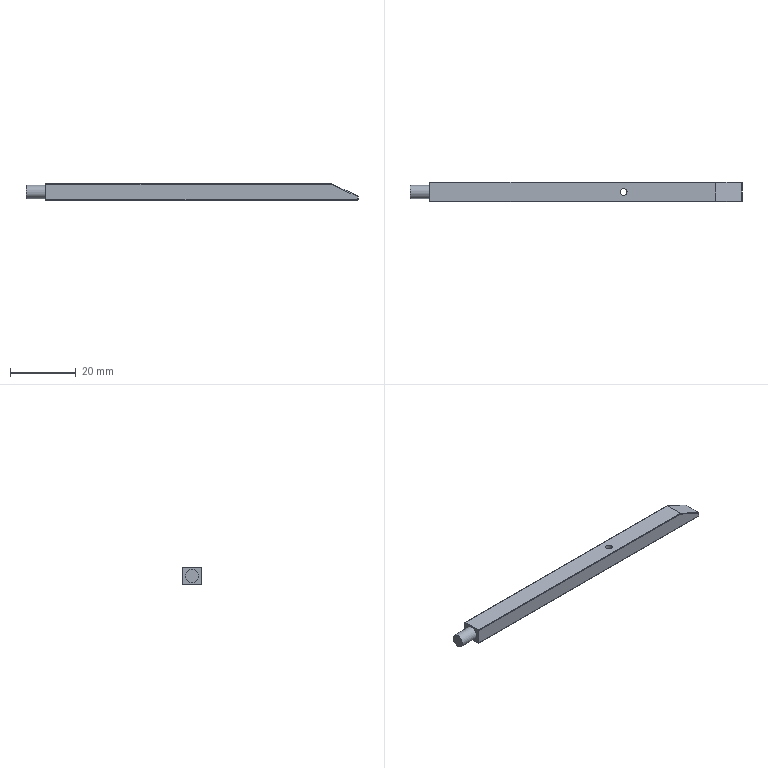Part | STEP file | 1-08.2 | 1 solid | 24 faces | box 101 x 6 x 5 mm | volume 2812 mm3 | plane 22 | cylinder 2 | commonest cylinder face diameters 2 x1 4 x1
STEP:
#1=CARTESIAN_POINT('',(0.,0.,0.));
#2=DIRECTION('',(0.,0.,1.));
#3=DIRECTION('',(1.,0.,0.));
#4=AXIS2_PLACEMENT_3D('',#1,#2,#3);
#5=CARTESIAN_POINT('',(-43.5,-2.,0.));
#6=VERTEX_POINT('',#5);
#7=CARTESIAN_POINT('',(-43.5,0.,0.));
#8=DIRECTION('',(-1.,0.,0.));
#9=DIRECTION('',(0.,-1.,0.));
#10=AXIS2_PLACEMENT_3D('',#7,#8,#9);
#11=CIRCLE('',#10,2.);
#12=CARTESIAN_POINT('',(-43.5,0.,0.));
#13=DIRECTION('',(-1.,0.,0.));
#14=DIRECTION('',(0.,-1.,0.));
#15=AXIS2_PLACEMENT_3D('',#12,#13,#14);
#16=CYLINDRICAL_SURFACE('',#15,2.);
#17=CARTESIAN_POINT('',(0.,0.));
#18=DIRECTION('',(1.,0.));
#19=VECTOR('',#18,1.);
#20=LINE('',#17,#19);
#21=(GEOMETRIC_REPRESENTATION_CONTEXT(2)PARAMETRIC_REPRESENTATION_CONTEXT()REPRESENTATION_CONTEXT('',''));
#22=DEFINITIONAL_REPRESENTATION('',(#20),#21);
#23=PCURVE('',#16,#22);
#24=CARTESIAN_POINT('',(-43.5,0.,0.));
#25=DIRECTION('',(1.,0.,0.));
#26=DIRECTION('',(0.,0.,-1.));
#27=AXIS2_PLACEMENT_3D('',#24,#25,#26);
#28=PLANE('',#27);
#29=CARTESIAN_POINT('',(0.,-2.));
#30=CARTESIAN_POINT('',(-3.464,-2.));
#31=CARTESIAN_POINT('',(-1.732,1.));
#32=CARTESIAN_POINT('',(0.,4.));
#33=CARTESIAN_POINT('',(1.732,1.));
#34=CARTESIAN_POINT('',(3.464,-2.));
#35=CARTESIAN_POINT('',(0.,-2.));
#36=(BOUNDED_CURVE()B_SPLINE_CURVE(2,(#29,#30,#31,#32,#33,#34,#35),.UNSPECIFIED.,.T.,.F.)B_SPLINE_CURVE_WITH_KNOTS((1,2,2,2,2,1),(-2.094,0.,2.094,4.189,6.283,8.378),.UNSPECIFIED.)CURVE()GEOMETRIC_REPRESENTATION_ITEM()RATIONAL_B_SPLINE_CURVE((1.,0.5,1.,0.5,1.,0.5,1.))REPRESENTATION_ITEM(''));
#37=(GEOMETRIC_REPRESENTATION_CONTEXT(2)PARAMETRIC_REPRESENTATION_CONTEXT()REPRESENTATION_CONTEXT('',''));
#38=DEFINITIONAL_REPRESENTATION('',(#36),#37);
#39=PCURVE('',#28,#38);
#40=SURFACE_CURVE('',#11,(#23,#39),.PCURVE_S1.);
#41=EDGE_CURVE('',#6,#6,#40,.T.);
#42=ORIENTED_EDGE('',*,*,#41,.T.);
#43=CARTESIAN_POINT('',(-49.5,-2.,0.));
#44=VERTEX_POINT('',#43);
#45=CARTESIAN_POINT('',(-43.5,-2.,0.));
#46=DIRECTION('',(-1.,0.,0.));
#47=VECTOR('',#46,1.);
#48=LINE('',#45,#47);
#49=CARTESIAN_POINT('',(6.283,0.));
#50=DIRECTION('',(0.,1.));
#51=VECTOR('',#50,1.);
#52=LINE('',#49,#51);
#53=(GEOMETRIC_REPRESENTATION_CONTEXT(2)PARAMETRIC_REPRESENTATION_CONTEXT()REPRESENTATION_CONTEXT('',''));
#54=DEFINITIONAL_REPRESENTATION('',(#52),#53);
#55=PCURVE('',#16,#54);
#56=CARTESIAN_POINT('',(0.,0.));
#57=DIRECTION('',(0.,1.));
#58=VECTOR('',#57,1.);
#59=LINE('',#56,#58);
#60=(GEOMETRIC_REPRESENTATION_CONTEXT(2)PARAMETRIC_REPRESENTATION_CONTEXT()REPRESENTATION_CONTEXT('',''));
#61=DEFINITIONAL_REPRESENTATION('',(#59),#60);
#62=PCURVE('',#16,#61);
#63=SEAM_CURVE('',#48,(#55,#62),.PCURVE_S1.);
#64=EDGE_CURVE('',#6,#44,#63,.T.);
#65=ORIENTED_EDGE('',*,*,#64,.T.);
#66=CARTESIAN_POINT('',(-49.5,0.,0.));
#67=DIRECTION('',(-1.,0.,0.));
#68=DIRECTION('',(0.,-1.,0.));
#69=AXIS2_PLACEMENT_3D('',#66,#67,#68);
#70=CIRCLE('',#69,2.);
#71=CARTESIAN_POINT('',(0.,6.));
#72=DIRECTION('',(1.,0.));
#73=VECTOR('',#72,1.);
#74=LINE('',#71,#73);
#75=(GEOMETRIC_REPRESENTATION_CONTEXT(2)PARAMETRIC_REPRESENTATION_CONTEXT()REPRESENTATION_CONTEXT('',''));
#76=DEFINITIONAL_REPRESENTATION('',(#74),#75);
#77=PCURVE('',#16,#76);
#78=CARTESIAN_POINT('',(-49.5,0.5359,0.));
#79=DIRECTION('',(-1.,0.,0.));
#80=DIRECTION('',(0.,-1.,0.));
#81=AXIS2_PLACEMENT_3D('',#78,#79,#80);
#82=PLANE('',#81);
#83=CARTESIAN_POINT('',(0.5359,0.));
#84=DIRECTION('',(1.,0.));
#85=AXIS2_PLACEMENT_2D('',#83,#84);
#86=CIRCLE('',#85,2.);
#87=(GEOMETRIC_REPRESENTATION_CONTEXT(2)PARAMETRIC_REPRESENTATION_CONTEXT()REPRESENTATION_CONTEXT('',''));
#88=DEFINITIONAL_REPRESENTATION('',(#86),#87);
#89=PCURVE('',#82,#88);
#90=SURFACE_CURVE('',#70,(#77,#89),.PCURVE_S1.);
#91=EDGE_CURVE('',#44,#44,#90,.T.);
#92=ORIENTED_EDGE('',*,*,#91,.F.);
#93=ORIENTED_EDGE('',*,*,#64,.F.);
#94=EDGE_LOOP('',(#42,#65,#92,#93));
#95=FACE_BOUND('',#94,.T.);
#96=ADVANCED_FACE('',(#95),#16,.T.);
#97=ORIENTED_EDGE('',*,*,#91,.T.);
#98=EDGE_LOOP('',(#97));
#99=FACE_BOUND('',#98,.T.);
#100=ADVANCED_FACE('',(#99),#82,.T.);
#101=CARTESIAN_POINT('',(-43.5,-3.,2.3));
#102=VERTEX_POINT('',#101);
#103=CARTESIAN_POINT('',(-43.5,-3.,-2.3));
#104=VERTEX_POINT('',#103);
#105=CARTESIAN_POINT('',(-43.5,-3.,2.3));
#106=DIRECTION('',(0.,0.,-1.));
#107=VECTOR('',#106,1.);
#108=LINE('',#105,#107);
#109=CARTESIAN_POINT('',(4.,-3.,45.));
#110=DIRECTION('',(0.,-1.,0.));
#111=DIRECTION('',(1.,0.,0.));
#112=AXIS2_PLACEMENT_3D('',#109,#110,#111);
#113=PLANE('',#112);
#114=CARTESIAN_POINT('',(-47.5,-42.7));
#115=DIRECTION('',(0.,-1.));
#116=VECTOR('',#115,1.);
#117=LINE('',#114,#116);
#118=(GEOMETRIC_REPRESENTATION_CONTEXT(2)PARAMETRIC_REPRESENTATION_CONTEXT()REPRESENTATION_CONTEXT('',''));
#119=DEFINITIONAL_REPRESENTATION('',(#117),#118);
#120=PCURVE('',#113,#119);
#121=CARTESIAN_POINT('',(-2.3,-3.));
#122=DIRECTION('',(1.,0.));
#123=VECTOR('',#122,1.);
#124=LINE('',#121,#123);
#125=(GEOMETRIC_REPRESENTATION_CONTEXT(2)PARAMETRIC_REPRESENTATION_CONTEXT()REPRESENTATION_CONTEXT('',''));
#126=DEFINITIONAL_REPRESENTATION('',(#124),#125);
#127=PCURVE('',#28,#126);
#128=SURFACE_CURVE('',#108,(#120,#127),.PCURVE_S1.);
#129=EDGE_CURVE('',#102,#104,#128,.T.);
#130=ORIENTED_EDGE('',*,*,#129,.T.);
#131=CARTESIAN_POINT('',(51.3,-3.,-2.3));
#132=VERTEX_POINT('',#131);
#133=CARTESIAN_POINT('',(-43.5,-3.,-2.3));
#134=DIRECTION('',(1.,0.,0.));
#135=VECTOR('',#134,1.);
#136=LINE('',#133,#135);
#137=CARTESIAN_POINT('',(-47.5,-47.3));
#138=DIRECTION('',(1.,0.));
#139=VECTOR('',#138,1.);
#140=LINE('',#137,#139);
#141=(GEOMETRIC_REPRESENTATION_CONTEXT(2)PARAMETRIC_REPRESENTATION_CONTEXT()REPRESENTATION_CONTEXT('',''));
#142=DEFINITIONAL_REPRESENTATION('',(#140),#141);
#143=PCURVE('',#113,#142);
#144=CARTESIAN_POINT('',(4.,-2.9,-2.4));
#145=DIRECTION('',(0.,-0.7071,-0.7071));
#146=DIRECTION('',(0.,0.7071,-0.7071));
#147=AXIS2_PLACEMENT_3D('',#144,#145,#146);
#148=PLANE('',#147);
#149=CARTESIAN_POINT('',(-0.1414,-47.5));
#150=DIRECTION('',(0.,1.));
#151=VECTOR('',#150,1.);
#152=LINE('',#149,#151);
#153=(GEOMETRIC_REPRESENTATION_CONTEXT(2)PARAMETRIC_REPRESENTATION_CONTEXT()REPRESENTATION_CONTEXT('',''));
#154=DEFINITIONAL_REPRESENTATION('',(#152),#153);
#155=PCURVE('',#148,#154);
#156=SURFACE_CURVE('',#136,(#143,#155),.PCURVE_S1.);
#157=EDGE_CURVE('',#104,#132,#156,.T.);
#158=ORIENTED_EDGE('',*,*,#157,.T.);
#159=CARTESIAN_POINT('',(51.3,-3.,-1.43));
#160=VERTEX_POINT('',#159);
#161=CARTESIAN_POINT('',(51.3,-3.,-2.3));
#162=DIRECTION('',(0.,0.,1.));
#163=VECTOR('',#162,1.);
#164=LINE('',#161,#163);
#165=CARTESIAN_POINT('',(47.3,-47.3));
#166=DIRECTION('',(0.,1.));
#167=VECTOR('',#166,1.);
#168=LINE('',#165,#167);
#169=(GEOMETRIC_REPRESENTATION_CONTEXT(2)PARAMETRIC_REPRESENTATION_CONTEXT()REPRESENTATION_CONTEXT('',''));
#170=DEFINITIONAL_REPRESENTATION('',(#168),#169);
#171=PCURVE('',#113,#170);
#172=CARTESIAN_POINT('',(51.4,-2.9,0.1745));
#173=DIRECTION('',(0.7071,-0.7071,0.));
#174=DIRECTION('',(0.7071,0.7071,0.));
#175=AXIS2_PLACEMENT_3D('',#172,#173,#174);
#176=PLANE('',#175);
#177=CARTESIAN_POINT('',(-0.1414,-2.474));
#178=DIRECTION('',(0.,1.));
#179=VECTOR('',#178,1.);
#180=LINE('',#177,#179);
#181=(GEOMETRIC_REPRESENTATION_CONTEXT(2)PARAMETRIC_REPRESENTATION_CONTEXT()REPRESENTATION_CONTEXT('',''));
#182=DEFINITIONAL_REPRESENTATION('',(#180),#181);
#183=PCURVE('',#176,#182);
#184=SURFACE_CURVE('',#164,(#171,#183),.PCURVE_S1.);
#185=EDGE_CURVE('',#132,#160,#184,.T.);
#186=ORIENTED_EDGE('',*,*,#185,.T.);
#187=CARTESIAN_POINT('',(51.234,-3.,-1.327));
#188=VERTEX_POINT('',#187);
#189=CARTESIAN_POINT('',(51.234,-3.,-1.327));
#190=DIRECTION('',(0.5373,0.,-0.8434));
#191=VECTOR('',#190,1.);
#192=LINE('',#189,#191);
#193=CARTESIAN_POINT('',(47.234,-46.327));
#194=DIRECTION('',(0.5373,-0.8434));
#195=VECTOR('',#194,1.);
#196=LINE('',#193,#195);
#197=(GEOMETRIC_REPRESENTATION_CONTEXT(2)PARAMETRIC_REPRESENTATION_CONTEXT()REPRESENTATION_CONTEXT('',''));
#198=DEFINITIONAL_REPRESENTATION('',(#196),#197);
#199=PCURVE('',#113,#198);
#200=CARTESIAN_POINT('',(51.343,-2.876,-1.303));
#201=DIRECTION('',(0.6447,-0.6447,0.4107));
#202=DIRECTION('',(-0.7071,-0.7071,0.));
#203=AXIS2_PLACEMENT_3D('',#200,#201,#202);
#204=PLANE('',#203);
#205=CARTESIAN_POINT('',(0.1647,0.02601));
#206=DIRECTION('',(-0.3799,0.925));
#207=VECTOR('',#206,1.);
#208=LINE('',#205,#207);
#209=(GEOMETRIC_REPRESENTATION_CONTEXT(2)PARAMETRIC_REPRESENTATION_CONTEXT()REPRESENTATION_CONTEXT('',''));
#210=DEFINITIONAL_REPRESENTATION('',(#208),#209);
#211=PCURVE('',#204,#210);
#212=SURFACE_CURVE('',#192,(#199,#211),.PCURVE_S1.);
#213=EDGE_CURVE('',#188,#160,#212,.T.);
#214=ORIENTED_EDGE('',*,*,#213,.F.);
#215=CARTESIAN_POINT('',(43.456,-3.,2.3));
#216=VERTEX_POINT('',#215);
#217=CARTESIAN_POINT('',(51.234,-3.,-1.327));
#218=DIRECTION('',(-0.9063,0.,0.4226));
#219=VECTOR('',#218,1.);
#220=LINE('',#217,#219);
#221=CARTESIAN_POINT('',(47.234,-46.327));
#222=DIRECTION('',(-0.9063,0.4226));
#223=VECTOR('',#222,1.);
#224=LINE('',#221,#223);
#225=(GEOMETRIC_REPRESENTATION_CONTEXT(2)PARAMETRIC_REPRESENTATION_CONTEXT()REPRESENTATION_CONTEXT('',''));
#226=DEFINITIONAL_REPRESENTATION('',(#224),#225);
#227=PCURVE('',#113,#226);
#228=CARTESIAN_POINT('',(47.458,-2.9,0.5441));
#229=DIRECTION('',(0.2988,-0.7071,0.6409));
#230=DIRECTION('',(0.2988,0.7071,0.6409));
#231=AXIS2_PLACEMENT_3D('',#228,#229,#230);
#232=PLANE('',#231);
#233=CARTESIAN_POINT('',(-0.1414,-4.214));
#234=DIRECTION('',(0.,1.));
#235=VECTOR('',#234,1.);
#236=LINE('',#233,#235);
#237=(GEOMETRIC_REPRESENTATION_CONTEXT(2)PARAMETRIC_REPRESENTATION_CONTEXT()REPRESENTATION_CONTEXT('',''));
#238=DEFINITIONAL_REPRESENTATION('',(#236),#237);
#239=PCURVE('',#232,#238);
#240=SURFACE_CURVE('',#220,(#227,#239),.PCURVE_S1.);
#241=EDGE_CURVE('',#188,#216,#240,.T.);
#242=ORIENTED_EDGE('',*,*,#241,.T.);
#243=CARTESIAN_POINT('',(43.456,-3.,2.3));
#244=DIRECTION('',(-1.,0.,0.));
#245=VECTOR('',#244,1.);
#246=LINE('',#243,#245);
#247=CARTESIAN_POINT('',(39.456,-42.7));
#248=DIRECTION('',(-1.,0.));
#249=VECTOR('',#248,1.);
#250=LINE('',#247,#249);
#251=(GEOMETRIC_REPRESENTATION_CONTEXT(2)PARAMETRIC_REPRESENTATION_CONTEXT()REPRESENTATION_CONTEXT('',''));
#252=DEFINITIONAL_REPRESENTATION('',(#250),#251);
#253=PCURVE('',#113,#252);
#254=CARTESIAN_POINT('',(6.375,-2.9,2.4));
#255=DIRECTION('',(0.,-0.7071,0.7071));
#256=DIRECTION('',(0.,0.7071,0.7071));
#257=AXIS2_PLACEMENT_3D('',#254,#255,#256);
#258=PLANE('',#257);
#259=CARTESIAN_POINT('',(-0.1414,-37.081));
#260=DIRECTION('',(0.,1.));
#261=VECTOR('',#260,1.);
#262=LINE('',#259,#261);
#263=(GEOMETRIC_REPRESENTATION_CONTEXT(2)PARAMETRIC_REPRESENTATION_CONTEXT()REPRESENTATION_CONTEXT('',''));
#264=DEFINITIONAL_REPRESENTATION('',(#262),#263);
#265=PCURVE('',#258,#264);
#266=SURFACE_CURVE('',#246,(#253,#265),.PCURVE_S1.);
#267=EDGE_CURVE('',#216,#102,#266,.T.);
#268=ORIENTED_EDGE('',*,*,#267,.T.);
#269=EDGE_LOOP('',(#130,#158,#186,#214,#242,#268));
#270=FACE_BOUND('',#269,.T.);
#271=ADVANCED_FACE('',(#270),#113,.T.);
#272=CARTESIAN_POINT('',(-43.5,3.,2.3));
#273=VERTEX_POINT('',#272);
#274=CARTESIAN_POINT('',(-43.5,3.,-2.3));
#275=VERTEX_POINT('',#274);
#276=CARTESIAN_POINT('',(-43.5,3.,2.3));
#277=DIRECTION('',(0.,0.,-1.));
#278=VECTOR('',#277,1.);
#279=LINE('',#276,#278);
#280=CARTESIAN_POINT('',(4.,3.,45.));
#281=DIRECTION('',(0.,-1.,0.));
#282=DIRECTION('',(1.,0.,0.));
#283=AXIS2_PLACEMENT_3D('',#280,#281,#282);
#284=PLANE('',#283);
#285=CARTESIAN_POINT('',(-47.5,-42.7));
#286=DIRECTION('',(0.,-1.));
#287=VECTOR('',#286,1.);
#288=LINE('',#285,#287);
#289=(GEOMETRIC_REPRESENTATION_CONTEXT(2)PARAMETRIC_REPRESENTATION_CONTEXT()REPRESENTATION_CONTEXT('',''));
#290=DEFINITIONAL_REPRESENTATION('',(#288),#289);
#291=PCURVE('',#284,#290);
#292=CARTESIAN_POINT('',(-2.3,3.));
#293=DIRECTION('',(1.,0.));
#294=VECTOR('',#293,1.);
#295=LINE('',#292,#294);
#296=(GEOMETRIC_REPRESENTATION_CONTEXT(2)PARAMETRIC_REPRESENTATION_CONTEXT()REPRESENTATION_CONTEXT('',''));
#297=DEFINITIONAL_REPRESENTATION('',(#295),#296);
#298=PCURVE('',#28,#297);
#299=SURFACE_CURVE('',#279,(#291,#298),.PCURVE_S1.);
#300=EDGE_CURVE('',#273,#275,#299,.T.);
#301=ORIENTED_EDGE('',*,*,#300,.T.);
#302=CARTESIAN_POINT('',(51.3,3.,-2.3));
#303=VERTEX_POINT('',#302);
#304=CARTESIAN_POINT('',(-43.5,3.,-2.3));
#305=DIRECTION('',(1.,0.,0.));
#306=VECTOR('',#305,1.);
#307=LINE('',#304,#306);
#308=CARTESIAN_POINT('',(-47.5,-47.3));
#309=DIRECTION('',(1.,0.));
#310=VECTOR('',#309,1.);
#311=LINE('',#308,#310);
#312=(GEOMETRIC_REPRESENTATION_CONTEXT(2)PARAMETRIC_REPRESENTATION_CONTEXT()REPRESENTATION_CONTEXT('',''));
#313=DEFINITIONAL_REPRESENTATION('',(#311),#312);
#314=PCURVE('',#284,#313);
#315=CARTESIAN_POINT('',(4.,2.9,-2.4));
#316=DIRECTION('',(0.,-0.7071,0.7071));
#317=DIRECTION('',(0.,-0.7071,-0.7071));
#318=AXIS2_PLACEMENT_3D('',#315,#316,#317);
#319=PLANE('',#318);
#320=CARTESIAN_POINT('',(-0.1414,-47.5));
#321=DIRECTION('',(0.,1.));
#322=VECTOR('',#321,1.);
#323=LINE('',#320,#322);
#324=(GEOMETRIC_REPRESENTATION_CONTEXT(2)PARAMETRIC_REPRESENTATION_CONTEXT()REPRESENTATION_CONTEXT('',''));
#325=DEFINITIONAL_REPRESENTATION('',(#323),#324);
#326=PCURVE('',#319,#325);
#327=SURFACE_CURVE('',#307,(#314,#326),.PCURVE_S1.);
#328=EDGE_CURVE('',#275,#303,#327,.T.);
#329=ORIENTED_EDGE('',*,*,#328,.T.);
#330=CARTESIAN_POINT('',(51.3,3.,-1.43));
#331=VERTEX_POINT('',#330);
#332=CARTESIAN_POINT('',(51.3,3.,-2.3));
#333=DIRECTION('',(0.,0.,1.));
#334=VECTOR('',#333,1.);
#335=LINE('',#332,#334);
#336=CARTESIAN_POINT('',(47.3,-47.3));
#337=DIRECTION('',(0.,1.));
#338=VECTOR('',#337,1.);
#339=LINE('',#336,#338);
#340=(GEOMETRIC_REPRESENTATION_CONTEXT(2)PARAMETRIC_REPRESENTATION_CONTEXT()REPRESENTATION_CONTEXT('',''));
#341=DEFINITIONAL_REPRESENTATION('',(#339),#340);
#342=PCURVE('',#284,#341);
#343=CARTESIAN_POINT('',(51.4,2.9,0.4556));
#344=DIRECTION('',(-0.7071,-0.7071,0.));
#345=DIRECTION('',(0.7071,-0.7071,0.));
#346=AXIS2_PLACEMENT_3D('',#343,#344,#345);
#347=PLANE('',#346);
#348=CARTESIAN_POINT('',(-0.1414,-2.756));
#349=DIRECTION('',(0.,1.));
#350=VECTOR('',#349,1.);
#351=LINE('',#348,#350);
#352=(GEOMETRIC_REPRESENTATION_CONTEXT(2)PARAMETRIC_REPRESENTATION_CONTEXT()REPRESENTATION_CONTEXT('',''));
#353=DEFINITIONAL_REPRESENTATION('',(#351),#352);
#354=PCURVE('',#347,#353);
#355=SURFACE_CURVE('',#335,(#342,#354),.PCURVE_S1.);
#356=EDGE_CURVE('',#303,#331,#355,.T.);
#357=ORIENTED_EDGE('',*,*,#356,.T.);
#358=CARTESIAN_POINT('',(51.234,3.,-1.327));
#359=VERTEX_POINT('',#358);
#360=CARTESIAN_POINT('',(51.234,3.,-1.327));
#361=DIRECTION('',(0.5373,0.,-0.8434));
#362=VECTOR('',#361,1.);
#363=LINE('',#360,#362);
#364=CARTESIAN_POINT('',(47.234,-46.327));
#365=DIRECTION('',(0.5373,-0.8434));
#366=VECTOR('',#365,1.);
#367=LINE('',#364,#366);
#368=(GEOMETRIC_REPRESENTATION_CONTEXT(2)PARAMETRIC_REPRESENTATION_CONTEXT()REPRESENTATION_CONTEXT('',''));
#369=DEFINITIONAL_REPRESENTATION('',(#367),#368);
#370=PCURVE('',#284,#369);
#371=CARTESIAN_POINT('',(51.343,2.876,-1.303));
#372=DIRECTION('',(-0.6447,-0.6447,-0.4107));
#373=DIRECTION('',(-0.7071,0.7071,0.));
#374=AXIS2_PLACEMENT_3D('',#371,#372,#373);
#375=PLANE('',#374);
#376=CARTESIAN_POINT('',(0.1647,0.02601));
#377=DIRECTION('',(-0.3799,0.925));
#378=VECTOR('',#377,1.);
#379=LINE('',#376,#378);
#380=(GEOMETRIC_REPRESENTATION_CONTEXT(2)PARAMETRIC_REPRESENTATION_CONTEXT()REPRESENTATION_CONTEXT('',''));
#381=DEFINITIONAL_REPRESENTATION('',(#379),#380);
#382=PCURVE('',#375,#381);
#383=SURFACE_CURVE('',#363,(#370,#382),.PCURVE_S1.);
#384=EDGE_CURVE('',#359,#331,#383,.T.);
#385=ORIENTED_EDGE('',*,*,#384,.F.);
#386=CARTESIAN_POINT('',(43.456,3.,2.3));
#387=VERTEX_POINT('',#386);
#388=CARTESIAN_POINT('',(51.234,3.,-1.327));
#389=DIRECTION('',(-0.9063,0.,0.4226));
#390=VECTOR('',#389,1.);
#391=LINE('',#388,#390);
#392=CARTESIAN_POINT('',(47.234,-46.327));
#393=DIRECTION('',(-0.9063,0.4226));
#394=VECTOR('',#393,1.);
#395=LINE('',#392,#394);
#396=(GEOMETRIC_REPRESENTATION_CONTEXT(2)PARAMETRIC_REPRESENTATION_CONTEXT()REPRESENTATION_CONTEXT('',''));
#397=DEFINITIONAL_REPRESENTATION('',(#395),#396);
#398=PCURVE('',#284,#397);
#399=CARTESIAN_POINT('',(47.458,2.9,0.5441));
#400=DIRECTION('',(-0.2988,-0.7071,-0.6409));
#401=DIRECTION('',(0.2988,-0.7071,0.6409));
#402=AXIS2_PLACEMENT_3D('',#399,#400,#401);
#403=PLANE('',#402);
#404=CARTESIAN_POINT('',(-0.1414,-4.214));
#405=DIRECTION('',(0.,1.));
#406=VECTOR('',#405,1.);
#407=LINE('',#404,#406);
#408=(GEOMETRIC_REPRESENTATION_CONTEXT(2)PARAMETRIC_REPRESENTATION_CONTEXT()REPRESENTATION_CONTEXT('',''));
#409=DEFINITIONAL_REPRESENTATION('',(#407),#408);
#410=PCURVE('',#403,#409);
#411=SURFACE_CURVE('',#391,(#398,#410),.PCURVE_S1.);
#412=EDGE_CURVE('',#359,#387,#411,.T.);
#413=ORIENTED_EDGE('',*,*,#412,.T.);
#414=CARTESIAN_POINT('',(43.456,3.,2.3));
#415=DIRECTION('',(-1.,0.,0.));
#416=VECTOR('',#415,1.);
#417=LINE('',#414,#416);
#418=CARTESIAN_POINT('',(39.456,-42.7));
#419=DIRECTION('',(-1.,0.));
#420=VECTOR('',#419,1.);
#421=LINE('',#418,#420);
#422=(GEOMETRIC_REPRESENTATION_CONTEXT(2)PARAMETRIC_REPRESENTATION_CONTEXT()REPRESENTATION_CONTEXT('',''));
#423=DEFINITIONAL_REPRESENTATION('',(#421),#422);
#424=PCURVE('',#284,#423);
#425=CARTESIAN_POINT('',(6.375,2.9,2.4));
#426=DIRECTION('',(0.,-0.7071,-0.7071));
#427=DIRECTION('',(0.,-0.7071,0.7071));
#428=AXIS2_PLACEMENT_3D('',#425,#426,#427);
#429=PLANE('',#428);
#430=CARTESIAN_POINT('',(-0.1414,-37.081));
#431=DIRECTION('',(0.,1.));
#432=VECTOR('',#431,1.);
#433=LINE('',#430,#432);
#434=(GEOMETRIC_REPRESENTATION_CONTEXT(2)PARAMETRIC_REPRESENTATION_CONTEXT()REPRESENTATION_CONTEXT('',''));
#435=DEFINITIONAL_REPRESENTATION('',(#433),#434);
#436=PCURVE('',#429,#435);
#437=SURFACE_CURVE('',#417,(#424,#436),.PCURVE_S1.);
#438=EDGE_CURVE('',#387,#273,#437,.T.);
#439=ORIENTED_EDGE('',*,*,#438,.T.);
#440=EDGE_LOOP('',(#301,#329,#357,#385,#413,#439));
#441=FACE_BOUND('',#440,.F.);
#442=ADVANCED_FACE('',(#441),#284,.F.);
#443=CARTESIAN_POINT('',(51.5,2.8,-2.3));
#444=VERTEX_POINT('',#443);
#445=CARTESIAN_POINT('',(51.5,2.8,-1.43));
#446=VERTEX_POINT('',#445);
#447=CARTESIAN_POINT('',(51.5,2.8,-2.3));
#448=DIRECTION('',(0.,0.,1.));
#449=VECTOR('',#448,1.);
#450=LINE('',#447,#449);
#451=CARTESIAN_POINT('',(51.5,0.,-1.865));
#452=DIRECTION('',(-1.,0.,0.));
#453=DIRECTION('',(0.,0.,1.));
#454=AXIS2_PLACEMENT_3D('',#451,#452,#453);
#455=PLANE('',#454);
#456=CARTESIAN_POINT('',(-0.4348,2.8));
#457=DIRECTION('',(1.,0.));
#458=VECTOR('',#457,1.);
#459=LINE('',#456,#458);
#460=(GEOMETRIC_REPRESENTATION_CONTEXT(2)PARAMETRIC_REPRESENTATION_CONTEXT()REPRESENTATION_CONTEXT('',''));
#461=DEFINITIONAL_REPRESENTATION('',(#459),#460);
#462=PCURVE('',#455,#461);
#463=CARTESIAN_POINT('',(0.1414,-2.756));
#464=DIRECTION('',(0.,1.));
#465=VECTOR('',#464,1.);
#466=LINE('',#463,#465);
#467=(GEOMETRIC_REPRESENTATION_CONTEXT(2)PARAMETRIC_REPRESENTATION_CONTEXT()REPRESENTATION_CONTEXT('',''));
#468=DEFINITIONAL_REPRESENTATION('',(#466),#467);
#469=PCURVE('',#347,#468);
#470=SURFACE_CURVE('',#450,(#462,#469),.PCURVE_S1.);
#471=EDGE_CURVE('',#444,#446,#470,.T.);
#472=ORIENTED_EDGE('',*,*,#471,.F.);
#473=CARTESIAN_POINT('',(51.5,-2.8,-2.3));
#474=VERTEX_POINT('',#473);
#475=CARTESIAN_POINT('',(51.5,-2.8,-2.3));
#476=DIRECTION('',(0.,1.,0.));
#477=VECTOR('',#476,1.);
#478=LINE('',#475,#477);
#479=CARTESIAN_POINT('',(-0.4348,-2.8));
#480=DIRECTION('',(0.,1.));
#481=VECTOR('',#480,1.);
#482=LINE('',#479,#481);
#483=(GEOMETRIC_REPRESENTATION_CONTEXT(2)PARAMETRIC_REPRESENTATION_CONTEXT()REPRESENTATION_CONTEXT('',''));
#484=DEFINITIONAL_REPRESENTATION('',(#482),#483);
#485=PCURVE('',#455,#484);
#486=CARTESIAN_POINT('',(51.4,0.,-2.4));
#487=DIRECTION('',(-0.7071,0.,0.7071));
#488=DIRECTION('',(0.7071,0.,0.7071));
#489=AXIS2_PLACEMENT_3D('',#486,#487,#488);
#490=PLANE('',#489);
#491=CARTESIAN_POINT('',(0.1414,-2.8));
#492=DIRECTION('',(0.,1.));
#493=VECTOR('',#492,1.);
#494=LINE('',#491,#493);
#495=(GEOMETRIC_REPRESENTATION_CONTEXT(2)PARAMETRIC_REPRESENTATION_CONTEXT()REPRESENTATION_CONTEXT('',''));
#496=DEFINITIONAL_REPRESENTATION('',(#494),#495);
#497=PCURVE('',#490,#496);
#498=SURFACE_CURVE('',#478,(#485,#497),.PCURVE_S1.);
#499=EDGE_CURVE('',#474,#444,#498,.T.);
#500=ORIENTED_EDGE('',*,*,#499,.F.);
#501=CARTESIAN_POINT('',(51.5,-2.8,-1.43));
#502=VERTEX_POINT('',#501);
#503=CARTESIAN_POINT('',(51.5,-2.8,-2.3));
#504=DIRECTION('',(0.,0.,1.));
#505=VECTOR('',#504,1.);
#506=LINE('',#503,#505);
#507=CARTESIAN_POINT('',(-0.4348,-2.8));
#508=DIRECTION('',(1.,0.));
#509=VECTOR('',#508,1.);
#510=LINE('',#507,#509);
#511=(GEOMETRIC_REPRESENTATION_CONTEXT(2)PARAMETRIC_REPRESENTATION_CONTEXT()REPRESENTATION_CONTEXT('',''));
#512=DEFINITIONAL_REPRESENTATION('',(#510),#511);
#513=PCURVE('',#455,#512);
#514=CARTESIAN_POINT('',(0.1414,-2.474));
#515=DIRECTION('',(0.,1.));
#516=VECTOR('',#515,1.);
#517=LINE('',#514,#516);
#518=(GEOMETRIC_REPRESENTATION_CONTEXT(2)PARAMETRIC_REPRESENTATION_CONTEXT()REPRESENTATION_CONTEXT('',''));
#519=DEFINITIONAL_REPRESENTATION('',(#517),#518);
#520=PCURVE('',#176,#519);
#521=SURFACE_CURVE('',#506,(#513,#520),.PCURVE_S1.);
#522=EDGE_CURVE('',#474,#502,#521,.T.);
#523=ORIENTED_EDGE('',*,*,#522,.T.);
#524=CARTESIAN_POINT('',(51.5,-2.8,-1.43));
#525=DIRECTION('',(0.,1.,0.));
#526=VECTOR('',#525,1.);
#527=LINE('',#524,#526);
#528=CARTESIAN_POINT('',(0.4348,-2.8));
#529=DIRECTION('',(0.,1.));
#530=VECTOR('',#529,1.);
#531=LINE('',#528,#530);
#532=(GEOMETRIC_REPRESENTATION_CONTEXT(2)PARAMETRIC_REPRESENTATION_CONTEXT()REPRESENTATION_CONTEXT('',''));
#533=DEFINITIONAL_REPRESENTATION('',(#531),#532);
#534=PCURVE('',#455,#533);
#535=CARTESIAN_POINT('',(51.409,0.,-1.288));
#536=DIRECTION('',(-0.8434,0.,-0.5373));
#537=DIRECTION('',(-0.5373,0.,0.8434));
#538=AXIS2_PLACEMENT_3D('',#535,#536,#537);
#539=PLANE('',#538);
#540=CARTESIAN_POINT('',(-0.1687,-2.8));
#541=DIRECTION('',(0.,1.));
#542=VECTOR('',#541,1.);
#543=LINE('',#540,#542);
#544=(GEOMETRIC_REPRESENTATION_CONTEXT(2)PARAMETRIC_REPRESENTATION_CONTEXT()REPRESENTATION_CONTEXT('',''));
#545=DEFINITIONAL_REPRESENTATION('',(#543),#544);
#546=PCURVE('',#539,#545);
#547=SURFACE_CURVE('',#527,(#534,#546),.PCURVE_S1.);
#548=EDGE_CURVE('',#502,#446,#547,.T.);
#549=ORIENTED_EDGE('',*,*,#548,.T.);
#550=EDGE_LOOP('',(#472,#500,#523,#549));
#551=FACE_BOUND('',#550,.F.);
#552=ADVANCED_FACE('',(#551),#455,.F.);
#553=CARTESIAN_POINT('',(43.5,-2.8,2.5));
#554=VERTEX_POINT('',#553);
#555=CARTESIAN_POINT('',(43.5,2.8,2.5));
#556=VERTEX_POINT('',#555);
#557=CARTESIAN_POINT('',(43.5,-2.8,2.5));
#558=DIRECTION('',(0.,1.,0.));
#559=VECTOR('',#558,1.);
#560=LINE('',#557,#559);
#561=CARTESIAN_POINT('',(47.5,0.,0.6348));
#562=DIRECTION('',(-0.4226,0.,-0.9063));
#563=DIRECTION('',(-0.9063,0.,0.4226));
#564=AXIS2_PLACEMENT_3D('',#561,#562,#563);
#565=PLANE('',#564);
#566=CARTESIAN_POINT('',(4.414,-2.8));
#567=DIRECTION('',(0.,1.));
#568=VECTOR('',#567,1.);
#569=LINE('',#566,#568);
#570=(GEOMETRIC_REPRESENTATION_CONTEXT(2)PARAMETRIC_REPRESENTATION_CONTEXT()REPRESENTATION_CONTEXT('',''));
#571=DEFINITIONAL_REPRESENTATION('',(#569),#570);
#572=PCURVE('',#565,#571);
#573=CARTESIAN_POINT('',(0.,0.,2.5));
#574=DIRECTION('',(0.,0.,-1.));
#575=DIRECTION('',(-1.,0.,0.));
#576=AXIS2_PLACEMENT_3D('',#573,#574,#575);
#577=PLANE('',#576);
#578=CARTESIAN_POINT('',(-43.5,-2.8));
#579=DIRECTION('',(0.,1.));
#580=VECTOR('',#579,1.);
#581=LINE('',#578,#580);
#582=(GEOMETRIC_REPRESENTATION_CONTEXT(2)PARAMETRIC_REPRESENTATION_CONTEXT()REPRESENTATION_CONTEXT('',''));
#583=DEFINITIONAL_REPRESENTATION('',(#581),#582);
#584=PCURVE('',#577,#583);
#585=SURFACE_CURVE('',#560,(#572,#584),.PCURVE_S1.);
#586=EDGE_CURVE('',#554,#556,#585,.T.);
#587=ORIENTED_EDGE('',*,*,#586,.T.);
#588=CARTESIAN_POINT('',(51.319,2.8,-1.146));
#589=VERTEX_POINT('',#588);
#590=CARTESIAN_POINT('',(51.319,2.8,-1.146));
#591=DIRECTION('',(-0.9063,0.,0.4226));
#592=VECTOR('',#591,1.);
#593=LINE('',#590,#592);
#594=CARTESIAN_POINT('',(-4.214,2.8));
#595=DIRECTION('',(1.,0.));
#596=VECTOR('',#595,1.);
#597=LINE('',#594,#596);
#598=(GEOMETRIC_REPRESENTATION_CONTEXT(2)PARAMETRIC_REPRESENTATION_CONTEXT()REPRESENTATION_CONTEXT('',''));
#599=DEFINITIONAL_REPRESENTATION('',(#597),#598);
#600=PCURVE('',#565,#599);
#601=CARTESIAN_POINT('',(0.1414,-4.214));
#602=DIRECTION('',(0.,1.));
#603=VECTOR('',#602,1.);
#604=LINE('',#601,#603);
#605=(GEOMETRIC_REPRESENTATION_CONTEXT(2)PARAMETRIC_REPRESENTATION_CONTEXT()REPRESENTATION_CONTEXT('',''));
#606=DEFINITIONAL_REPRESENTATION('',(#604),#605);
#607=PCURVE('',#403,#606);
#608=SURFACE_CURVE('',#593,(#600,#607),.PCURVE_S1.);
#609=EDGE_CURVE('',#589,#556,#608,.T.);
#610=ORIENTED_EDGE('',*,*,#609,.F.);
#611=CARTESIAN_POINT('',(51.319,-2.8,-1.146));
#612=VERTEX_POINT('',#611);
#613=CARTESIAN_POINT('',(51.319,-2.8,-1.146));
#614=DIRECTION('',(0.,1.,0.));
#615=VECTOR('',#614,1.);
#616=LINE('',#613,#615);
#617=CARTESIAN_POINT('',(-4.214,-2.8));
#618=DIRECTION('',(0.,1.));
#619=VECTOR('',#618,1.);
#620=LINE('',#617,#619);
#621=(GEOMETRIC_REPRESENTATION_CONTEXT(2)PARAMETRIC_REPRESENTATION_CONTEXT()REPRESENTATION_CONTEXT('',''));
#622=DEFINITIONAL_REPRESENTATION('',(#620),#621);
#623=PCURVE('',#565,#622);
#624=CARTESIAN_POINT('',(0.1687,-2.8));
#625=DIRECTION('',(0.,1.));
#626=VECTOR('',#625,1.);
#627=LINE('',#624,#626);
#628=(GEOMETRIC_REPRESENTATION_CONTEXT(2)PARAMETRIC_REPRESENTATION_CONTEXT()REPRESENTATION_CONTEXT('',''));
#629=DEFINITIONAL_REPRESENTATION('',(#627),#628);
#630=PCURVE('',#539,#629);
#631=SURFACE_CURVE('',#616,(#623,#630),.PCURVE_S1.);
#632=EDGE_CURVE('',#612,#589,#631,.T.);
#633=ORIENTED_EDGE('',*,*,#632,.F.);
#634=CARTESIAN_POINT('',(51.319,-2.8,-1.146));
#635=DIRECTION('',(-0.9063,0.,0.4226));
#636=VECTOR('',#635,1.);
#637=LINE('',#634,#636);
#638=CARTESIAN_POINT('',(-4.214,-2.8));
#639=DIRECTION('',(1.,0.));
#640=VECTOR('',#639,1.);
#641=LINE('',#638,#640);
#642=(GEOMETRIC_REPRESENTATION_CONTEXT(2)PARAMETRIC_REPRESENTATION_CONTEXT()REPRESENTATION_CONTEXT('',''));
#643=DEFINITIONAL_REPRESENTATION('',(#641),#642);
#644=PCURVE('',#565,#643);
#645=CARTESIAN_POINT('',(0.1414,-4.214));
#646=DIRECTION('',(0.,1.));
#647=VECTOR('',#646,1.);
#648=LINE('',#645,#647);
#649=(GEOMETRIC_REPRESENTATION_CONTEXT(2)PARAMETRIC_REPRESENTATION_CONTEXT()REPRESENTATION_CONTEXT('',''));
#650=DEFINITIONAL_REPRESENTATION('',(#648),#649);
#651=PCURVE('',#232,#650);
#652=SURFACE_CURVE('',#637,(#644,#651),.PCURVE_S1.);
#653=EDGE_CURVE('',#612,#554,#652,.T.);
#654=ORIENTED_EDGE('',*,*,#653,.T.);
#655=EDGE_LOOP('',(#587,#610,#633,#654));
#656=FACE_BOUND('',#655,.F.);
#657=ADVANCED_FACE('',(#656),#565,.F.);
#658=ORIENTED_EDGE('',*,*,#129,.T.);
#659=CARTESIAN_POINT('',(-43.5,-2.8,-2.5));
#660=VERTEX_POINT('',#659);
#661=CARTESIAN_POINT('',(-43.5,-3.,-2.3));
#662=DIRECTION('',(0.,0.7071,-0.7071));
#663=VECTOR('',#662,1.);
#664=LINE('',#661,#663);
#665=CARTESIAN_POINT('',(2.3,-3.));
#666=DIRECTION('',(0.7071,0.7071));
#667=VECTOR('',#666,1.);
#668=LINE('',#665,#667);
#669=(GEOMETRIC_REPRESENTATION_CONTEXT(2)PARAMETRIC_REPRESENTATION_CONTEXT()REPRESENTATION_CONTEXT('',''));
#670=DEFINITIONAL_REPRESENTATION('',(#668),#669);
#671=PCURVE('',#28,#670);
#672=CARTESIAN_POINT('',(-0.1414,-47.5));
#673=DIRECTION('',(1.,0.));
#674=VECTOR('',#673,1.);
#675=LINE('',#672,#674);
#676=(GEOMETRIC_REPRESENTATION_CONTEXT(2)PARAMETRIC_REPRESENTATION_CONTEXT()REPRESENTATION_CONTEXT('',''));
#677=DEFINITIONAL_REPRESENTATION('',(#675),#676);
#678=PCURVE('',#148,#677);
#679=SURFACE_CURVE('',#664,(#671,#678),.PCURVE_S1.);
#680=EDGE_CURVE('',#104,#660,#679,.T.);
#681=ORIENTED_EDGE('',*,*,#680,.T.);
#682=CARTESIAN_POINT('',(-43.5,2.8,-2.5));
#683=VERTEX_POINT('',#682);
#684=CARTESIAN_POINT('',(-43.5,-2.8,-2.5));
#685=DIRECTION('',(0.,1.,0.));
#686=VECTOR('',#685,1.);
#687=LINE('',#684,#686);
#688=CARTESIAN_POINT('',(2.5,-2.8));
#689=DIRECTION('',(0.,1.));
#690=VECTOR('',#689,1.);
#691=LINE('',#688,#690);
#692=(GEOMETRIC_REPRESENTATION_CONTEXT(2)PARAMETRIC_REPRESENTATION_CONTEXT()REPRESENTATION_CONTEXT('',''));
#693=DEFINITIONAL_REPRESENTATION('',(#691),#692);
#694=PCURVE('',#28,#693);
#695=CARTESIAN_POINT('',(4.,0.,-2.5));
#696=DIRECTION('',(0.,0.,1.));
#697=DIRECTION('',(1.,0.,0.));
#698=AXIS2_PLACEMENT_3D('',#695,#696,#697);
#699=PLANE('',#698);
#700=CARTESIAN_POINT('',(-47.5,-2.8));
#701=DIRECTION('',(0.,1.));
#702=VECTOR('',#701,1.);
#703=LINE('',#700,#702);
#704=(GEOMETRIC_REPRESENTATION_CONTEXT(2)PARAMETRIC_REPRESENTATION_CONTEXT()REPRESENTATION_CONTEXT('',''));
#705=DEFINITIONAL_REPRESENTATION('',(#703),#704);
#706=PCURVE('',#699,#705);
#707=SURFACE_CURVE('',#687,(#694,#706),.PCURVE_S1.);
#708=EDGE_CURVE('',#660,#683,#707,.T.);
#709=ORIENTED_EDGE('',*,*,#708,.T.);
#710=CARTESIAN_POINT('',(-43.5,3.,-2.3));
#711=DIRECTION('',(0.,-0.7071,-0.7071));
#712=VECTOR('',#711,1.);
#713=LINE('',#710,#712);
#714=CARTESIAN_POINT('',(2.3,3.));
#715=DIRECTION('',(0.7071,-0.7071));
#716=VECTOR('',#715,1.);
#717=LINE('',#714,#716);
#718=(GEOMETRIC_REPRESENTATION_CONTEXT(2)PARAMETRIC_REPRESENTATION_CONTEXT()REPRESENTATION_CONTEXT('',''));
#719=DEFINITIONAL_REPRESENTATION('',(#717),#718);
#720=PCURVE('',#28,#719);
#721=CARTESIAN_POINT('',(-0.1414,-47.5));
#722=DIRECTION('',(1.,0.));
#723=VECTOR('',#722,1.);
#724=LINE('',#721,#723);
#725=(GEOMETRIC_REPRESENTATION_CONTEXT(2)PARAMETRIC_REPRESENTATION_CONTEXT()REPRESENTATION_CONTEXT('',''));
#726=DEFINITIONAL_REPRESENTATION('',(#724),#725);
#727=PCURVE('',#319,#726);
#728=SURFACE_CURVE('',#713,(#720,#727),.PCURVE_S1.);
#729=EDGE_CURVE('',#275,#683,#728,.T.);
#730=ORIENTED_EDGE('',*,*,#729,.F.);
#731=ORIENTED_EDGE('',*,*,#300,.F.);
#732=CARTESIAN_POINT('',(-43.5,2.8,2.5));
#733=VERTEX_POINT('',#732);
#734=CARTESIAN_POINT('',(-43.5,3.,2.3));
#735=DIRECTION('',(0.,-0.7071,0.7071));
#736=VECTOR('',#735,1.);
#737=LINE('',#734,#736);
#738=CARTESIAN_POINT('',(-2.3,3.));
#739=DIRECTION('',(-0.7071,-0.7071));
#740=VECTOR('',#739,1.);
#741=LINE('',#738,#740);
#742=(GEOMETRIC_REPRESENTATION_CONTEXT(2)PARAMETRIC_REPRESENTATION_CONTEXT()REPRESENTATION_CONTEXT('',''));
#743=DEFINITIONAL_REPRESENTATION('',(#741),#742);
#744=PCURVE('',#28,#743);
#745=CARTESIAN_POINT('',(-0.1414,49.875));
#746=DIRECTION('',(1.,0.));
#747=VECTOR('',#746,1.);
#748=LINE('',#745,#747);
#749=(GEOMETRIC_REPRESENTATION_CONTEXT(2)PARAMETRIC_REPRESENTATION_CONTEXT()REPRESENTATION_CONTEXT('',''));
#750=DEFINITIONAL_REPRESENTATION('',(#748),#749);
#751=PCURVE('',#429,#750);
#752=SURFACE_CURVE('',#737,(#744,#751),.PCURVE_S1.);
#753=EDGE_CURVE('',#273,#733,#752,.T.);
#754=ORIENTED_EDGE('',*,*,#753,.T.);
#755=CARTESIAN_POINT('',(-43.5,-2.8,2.5));
#756=VERTEX_POINT('',#755);
#757=CARTESIAN_POINT('',(-43.5,-2.8,2.5));
#758=DIRECTION('',(0.,1.,0.));
#759=VECTOR('',#758,1.);
#760=LINE('',#757,#759);
#761=CARTESIAN_POINT('',(-2.5,-2.8));
#762=DIRECTION('',(0.,1.));
#763=VECTOR('',#762,1.);
#764=LINE('',#761,#763);
#765=(GEOMETRIC_REPRESENTATION_CONTEXT(2)PARAMETRIC_REPRESENTATION_CONTEXT()REPRESENTATION_CONTEXT('',''));
#766=DEFINITIONAL_REPRESENTATION('',(#764),#765);
#767=PCURVE('',#28,#766);
#768=CARTESIAN_POINT('',(43.5,-2.8));
#769=DIRECTION('',(0.,1.));
#770=VECTOR('',#769,1.);
#771=LINE('',#768,#770);
#772=(GEOMETRIC_REPRESENTATION_CONTEXT(2)PARAMETRIC_REPRESENTATION_CONTEXT()REPRESENTATION_CONTEXT('',''));
#773=DEFINITIONAL_REPRESENTATION('',(#771),#772);
#774=PCURVE('',#577,#773);
#775=SURFACE_CURVE('',#760,(#767,#774),.PCURVE_S1.);
#776=EDGE_CURVE('',#756,#733,#775,.T.);
#777=ORIENTED_EDGE('',*,*,#776,.F.);
#778=CARTESIAN_POINT('',(-43.5,-3.,2.3));
#779=DIRECTION('',(0.,0.7071,0.7071));
#780=VECTOR('',#779,1.);
#781=LINE('',#778,#780);
#782=CARTESIAN_POINT('',(-2.3,-3.));
#783=DIRECTION('',(-0.7071,0.7071));
#784=VECTOR('',#783,1.);
#785=LINE('',#782,#784);
#786=(GEOMETRIC_REPRESENTATION_CONTEXT(2)PARAMETRIC_REPRESENTATION_CONTEXT()REPRESENTATION_CONTEXT('',''));
#787=DEFINITIONAL_REPRESENTATION('',(#785),#786);
#788=PCURVE('',#28,#787);
#789=CARTESIAN_POINT('',(-0.1414,49.875));
#790=DIRECTION('',(1.,0.));
#791=VECTOR('',#790,1.);
#792=LINE('',#789,#791);
#793=(GEOMETRIC_REPRESENTATION_CONTEXT(2)PARAMETRIC_REPRESENTATION_CONTEXT()REPRESENTATION_CONTEXT('',''));
#794=DEFINITIONAL_REPRESENTATION('',(#792),#793);
#795=PCURVE('',#258,#794);
#796=SURFACE_CURVE('',#781,(#788,#795),.PCURVE_S1.);
#797=EDGE_CURVE('',#102,#756,#796,.T.);
#798=ORIENTED_EDGE('',*,*,#797,.F.);
#799=EDGE_LOOP('',(#658,#681,#709,#730,#731,#754,#777,#798));
#800=FACE_BOUND('',#799,.F.);
#801=ORIENTED_EDGE('',*,*,#41,.T.);
#802=EDGE_LOOP('',(#801));
#803=FACE_BOUND('',#802,.F.);
#804=ADVANCED_FACE('',(#800,#803),#28,.F.);
#805=ORIENTED_EDGE('',*,*,#680,.T.);
#806=CARTESIAN_POINT('',(51.3,-2.8,-2.5));
#807=VERTEX_POINT('',#806);
#808=CARTESIAN_POINT('',(-43.5,-2.8,-2.5));
#809=DIRECTION('',(1.,0.,0.));
#810=VECTOR('',#809,1.);
#811=LINE('',#808,#810);
#812=CARTESIAN_POINT('',(0.1414,-47.5));
#813=DIRECTION('',(0.,1.));
#814=VECTOR('',#813,1.);
#815=LINE('',#812,#814);
#816=(GEOMETRIC_REPRESENTATION_CONTEXT(2)PARAMETRIC_REPRESENTATION_CONTEXT()REPRESENTATION_CONTEXT('',''));
#817=DEFINITIONAL_REPRESENTATION('',(#815),#816);
#818=PCURVE('',#148,#817);
#819=CARTESIAN_POINT('',(-47.5,-2.8));
#820=DIRECTION('',(1.,0.));
#821=VECTOR('',#820,1.);
#822=LINE('',#819,#821);
#823=(GEOMETRIC_REPRESENTATION_CONTEXT(2)PARAMETRIC_REPRESENTATION_CONTEXT()REPRESENTATION_CONTEXT('',''));
#824=DEFINITIONAL_REPRESENTATION('',(#822),#823);
#825=PCURVE('',#699,#824);
#826=SURFACE_CURVE('',#811,(#818,#825),.PCURVE_S1.);
#827=EDGE_CURVE('',#660,#807,#826,.T.);
#828=ORIENTED_EDGE('',*,*,#827,.T.);
#829=CARTESIAN_POINT('',(51.3,-3.,-2.3));
#830=DIRECTION('',(0.,0.7071,-0.7071));
#831=VECTOR('',#830,1.);
#832=LINE('',#829,#831);
#833=CARTESIAN_POINT('',(-0.1414,47.3));
#834=DIRECTION('',(1.,0.));
#835=VECTOR('',#834,1.);
#836=LINE('',#833,#835);
#837=(GEOMETRIC_REPRESENTATION_CONTEXT(2)PARAMETRIC_REPRESENTATION_CONTEXT()REPRESENTATION_CONTEXT('',''));
#838=DEFINITIONAL_REPRESENTATION('',(#836),#837);
#839=PCURVE('',#148,#838);
#840=CARTESIAN_POINT('',(51.415,-2.842,-2.342));
#841=DIRECTION('',(0.5774,-0.5774,-0.5774));
#842=DIRECTION('',(0.,0.7071,-0.7071));
#843=AXIS2_PLACEMENT_3D('',#840,#841,#842);
#844=PLANE('',#843);
#845=CARTESIAN_POINT('',(-0.1414,-0.1414));
#846=DIRECTION('',(1.,0.));
#847=VECTOR('',#846,1.);
#848=LINE('',#845,#847);
#849=(GEOMETRIC_REPRESENTATION_CONTEXT(2)PARAMETRIC_REPRESENTATION_CONTEXT()REPRESENTATION_CONTEXT('',''));
#850=DEFINITIONAL_REPRESENTATION('',(#848),#849);
#851=PCURVE('',#844,#850);
#852=SURFACE_CURVE('',#832,(#839,#851),.PCURVE_S1.);
#853=EDGE_CURVE('',#132,#807,#852,.T.);
#854=ORIENTED_EDGE('',*,*,#853,.F.);
#855=ORIENTED_EDGE('',*,*,#157,.F.);
#856=EDGE_LOOP('',(#805,#828,#854,#855));
#857=FACE_BOUND('',#856,.T.);
#858=ADVANCED_FACE('',(#857),#148,.T.);
#859=ORIENTED_EDGE('',*,*,#729,.T.);
#860=CARTESIAN_POINT('',(51.3,2.8,-2.5));
#861=VERTEX_POINT('',#860);
#862=CARTESIAN_POINT('',(-43.5,2.8,-2.5));
#863=DIRECTION('',(1.,0.,0.));
#864=VECTOR('',#863,1.);
#865=LINE('',#862,#864);
#866=CARTESIAN_POINT('',(0.1414,-47.5));
#867=DIRECTION('',(0.,1.));
#868=VECTOR('',#867,1.);
#869=LINE('',#866,#868);
#870=(GEOMETRIC_REPRESENTATION_CONTEXT(2)PARAMETRIC_REPRESENTATION_CONTEXT()REPRESENTATION_CONTEXT('',''));
#871=DEFINITIONAL_REPRESENTATION('',(#869),#870);
#872=PCURVE('',#319,#871);
#873=CARTESIAN_POINT('',(-47.5,2.8));
#874=DIRECTION('',(1.,0.));
#875=VECTOR('',#874,1.);
#876=LINE('',#873,#875);
#877=(GEOMETRIC_REPRESENTATION_CONTEXT(2)PARAMETRIC_REPRESENTATION_CONTEXT()REPRESENTATION_CONTEXT('',''));
#878=DEFINITIONAL_REPRESENTATION('',(#876),#877);
#879=PCURVE('',#699,#878);
#880=SURFACE_CURVE('',#865,(#872,#879),.PCURVE_S1.);
#881=EDGE_CURVE('',#683,#861,#880,.T.);
#882=ORIENTED_EDGE('',*,*,#881,.T.);
#883=CARTESIAN_POINT('',(51.3,3.,-2.3));
#884=DIRECTION('',(0.,-0.7071,-0.7071));
#885=VECTOR('',#884,1.);
#886=LINE('',#883,#885);
#887=CARTESIAN_POINT('',(-0.1414,47.3));
#888=DIRECTION('',(1.,0.));
#889=VECTOR('',#888,1.);
#890=LINE('',#887,#889);
#891=(GEOMETRIC_REPRESENTATION_CONTEXT(2)PARAMETRIC_REPRESENTATION_CONTEXT()REPRESENTATION_CONTEXT('',''));
#892=DEFINITIONAL_REPRESENTATION('',(#890),#891);
#893=PCURVE('',#319,#892);
#894=CARTESIAN_POINT('',(51.415,2.842,-2.342));
#895=DIRECTION('',(-0.5774,-0.5774,0.5774));
#896=DIRECTION('',(0.,-0.7071,-0.7071));
#897=AXIS2_PLACEMENT_3D('',#894,#895,#896);
#898=PLANE('',#897);
#899=CARTESIAN_POINT('',(-0.1414,-0.1414));
#900=DIRECTION('',(1.,0.));
#901=VECTOR('',#900,1.);
#902=LINE('',#899,#901);
#903=(GEOMETRIC_REPRESENTATION_CONTEXT(2)PARAMETRIC_REPRESENTATION_CONTEXT()REPRESENTATION_CONTEXT('',''));
#904=DEFINITIONAL_REPRESENTATION('',(#902),#903);
#905=PCURVE('',#898,#904);
#906=SURFACE_CURVE('',#886,(#893,#905),.PCURVE_S1.);
#907=EDGE_CURVE('',#303,#861,#906,.T.);
#908=ORIENTED_EDGE('',*,*,#907,.F.);
#909=ORIENTED_EDGE('',*,*,#328,.F.);
#910=EDGE_LOOP('',(#859,#882,#908,#909));
#911=FACE_BOUND('',#910,.F.);
#912=ADVANCED_FACE('',(#911),#319,.F.);
#913=ORIENTED_EDGE('',*,*,#753,.F.);
#914=ORIENTED_EDGE('',*,*,#438,.F.);
#915=CARTESIAN_POINT('',(43.5,2.8,2.5));
#916=DIRECTION('',(-0.1549,0.6986,-0.6986));
#917=VECTOR('',#916,1.);
#918=LINE('',#915,#917);
#919=CARTESIAN_POINT('',(0.1414,-37.125));
#920=DIRECTION('',(-0.9879,0.1549));
#921=VECTOR('',#920,1.);
#922=LINE('',#919,#921);
#923=(GEOMETRIC_REPRESENTATION_CONTEXT(2)PARAMETRIC_REPRESENTATION_CONTEXT()REPRESENTATION_CONTEXT('',''));
#924=DEFINITIONAL_REPRESENTATION('',(#922),#923);
#925=PCURVE('',#429,#924);
#926=CARTESIAN_POINT('',(0.1414,4.414));
#927=DIRECTION('',(-0.9879,-0.1549));
#928=VECTOR('',#927,1.);
#929=LINE('',#926,#928);
#930=(GEOMETRIC_REPRESENTATION_CONTEXT(2)PARAMETRIC_REPRESENTATION_CONTEXT()REPRESENTATION_CONTEXT('',''));
#931=DEFINITIONAL_REPRESENTATION('',(#929),#930);
#932=PCURVE('',#403,#931);
#933=SURFACE_CURVE('',#918,(#925,#932),.PCURVE_S1.);
#934=EDGE_CURVE('',#556,#387,#933,.T.);
#935=ORIENTED_EDGE('',*,*,#934,.F.);
#936=CARTESIAN_POINT('',(43.5,2.8,2.5));
#937=DIRECTION('',(-1.,0.,0.));
#938=VECTOR('',#937,1.);
#939=LINE('',#936,#938);
#940=CARTESIAN_POINT('',(0.1414,-37.125));
#941=DIRECTION('',(0.,1.));
#942=VECTOR('',#941,1.);
#943=LINE('',#940,#942);
#944=(GEOMETRIC_REPRESENTATION_CONTEXT(2)PARAMETRIC_REPRESENTATION_CONTEXT()REPRESENTATION_CONTEXT('',''));
#945=DEFINITIONAL_REPRESENTATION('',(#943),#944);
#946=PCURVE('',#429,#945);
#947=CARTESIAN_POINT('',(-43.5,2.8));
#948=DIRECTION('',(1.,0.));
#949=VECTOR('',#948,1.);
#950=LINE('',#947,#949);
#951=(GEOMETRIC_REPRESENTATION_CONTEXT(2)PARAMETRIC_REPRESENTATION_CONTEXT()REPRESENTATION_CONTEXT('',''));
#952=DEFINITIONAL_REPRESENTATION('',(#950),#951);
#953=PCURVE('',#577,#952);
#954=SURFACE_CURVE('',#939,(#946,#953),.PCURVE_S1.);
#955=EDGE_CURVE('',#556,#733,#954,.T.);
#956=ORIENTED_EDGE('',*,*,#955,.T.);
#957=EDGE_LOOP('',(#913,#914,#935,#956));
#958=FACE_BOUND('',#957,.F.);
#959=ADVANCED_FACE('',(#958),#429,.F.);
#960=ORIENTED_EDGE('',*,*,#797,.F.);
#961=ORIENTED_EDGE('',*,*,#267,.F.);
#962=CARTESIAN_POINT('',(43.5,-2.8,2.5));
#963=DIRECTION('',(-0.1549,-0.6986,-0.6986));
#964=VECTOR('',#963,1.);
#965=LINE('',#962,#964);
#966=CARTESIAN_POINT('',(0.1414,-37.125));
#967=DIRECTION('',(-0.9879,0.1549));
#968=VECTOR('',#967,1.);
#969=LINE('',#966,#968);
#970=(GEOMETRIC_REPRESENTATION_CONTEXT(2)PARAMETRIC_REPRESENTATION_CONTEXT()REPRESENTATION_CONTEXT('',''));
#971=DEFINITIONAL_REPRESENTATION('',(#969),#970);
#972=PCURVE('',#258,#971);
#973=CARTESIAN_POINT('',(0.1414,4.414));
#974=DIRECTION('',(-0.9879,-0.1549));
#975=VECTOR('',#974,1.);
#976=LINE('',#973,#975);
#977=(GEOMETRIC_REPRESENTATION_CONTEXT(2)PARAMETRIC_REPRESENTATION_CONTEXT()REPRESENTATION_CONTEXT('',''));
#978=DEFINITIONAL_REPRESENTATION('',(#976),#977);
#979=PCURVE('',#232,#978);
#980=SURFACE_CURVE('',#965,(#972,#979),.PCURVE_S1.);
#981=EDGE_CURVE('',#554,#216,#980,.T.);
#982=ORIENTED_EDGE('',*,*,#981,.F.);
#983=CARTESIAN_POINT('',(43.5,-2.8,2.5));
#984=DIRECTION('',(-1.,0.,0.));
#985=VECTOR('',#984,1.);
#986=LINE('',#983,#985);
#987=CARTESIAN_POINT('',(0.1414,-37.125));
#988=DIRECTION('',(0.,1.));
#989=VECTOR('',#988,1.);
#990=LINE('',#987,#989);
#991=(GEOMETRIC_REPRESENTATION_CONTEXT(2)PARAMETRIC_REPRESENTATION_CONTEXT()REPRESENTATION_CONTEXT('',''));
#992=DEFINITIONAL_REPRESENTATION('',(#990),#991);
#993=PCURVE('',#258,#992);
#994=CARTESIAN_POINT('',(-43.5,-2.8));
#995=DIRECTION('',(1.,0.));
#996=VECTOR('',#995,1.);
#997=LINE('',#994,#996);
#998=(GEOMETRIC_REPRESENTATION_CONTEXT(2)PARAMETRIC_REPRESENTATION_CONTEXT()REPRESENTATION_CONTEXT('',''));
#999=DEFINITIONAL_REPRESENTATION('',(#997),#998);
#1000=PCURVE('',#577,#999);
#1001=SURFACE_CURVE('',#986,(#993,#1000),.PCURVE_S1.);
#1002=EDGE_CURVE('',#554,#756,#1001,.T.);
#1003=ORIENTED_EDGE('',*,*,#1002,.T.);
#1004=EDGE_LOOP('',(#960,#961,#982,#1003));
#1005=FACE_BOUND('',#1004,.T.);
#1006=ADVANCED_FACE('',(#1005),#258,.T.);
#1007=ORIENTED_EDGE('',*,*,#522,.T.);
#1008=CARTESIAN_POINT('',(51.3,-3.,-1.43));
#1009=DIRECTION('',(0.7071,0.7071,0.));
#1010=VECTOR('',#1009,1.);
#1011=LINE('',#1008,#1010);
#1012=CARTESIAN_POINT('',(-0.1414,-1.605));
#1013=DIRECTION('',(1.,0.));
#1014=VECTOR('',#1013,1.);
#1015=LINE('',#1012,#1014);
#1016=(GEOMETRIC_REPRESENTATION_CONTEXT(2)PARAMETRIC_REPRESENTATION_CONTEXT()REPRESENTATION_CONTEXT('',''));
#1017=DEFINITIONAL_REPRESENTATION('',(#1015),#1016);
#1018=PCURVE('',#176,#1017);
#1019=CARTESIAN_POINT('',(0.1182,0.1393));
#1020=DIRECTION('',(-1.,0.));
#1021=VECTOR('',#1020,1.);
#1022=LINE('',#1019,#1021);
#1023=(GEOMETRIC_REPRESENTATION_CONTEXT(2)PARAMETRIC_REPRESENTATION_CONTEXT()REPRESENTATION_CONTEXT('',''));
#1024=DEFINITIONAL_REPRESENTATION('',(#1022),#1023);
#1025=PCURVE('',#204,#1024);
#1026=SURFACE_CURVE('',#1011,(#1018,#1025),.PCURVE_S1.);
#1027=EDGE_CURVE('',#160,#502,#1026,.T.);
#1028=ORIENTED_EDGE('',*,*,#1027,.F.);
#1029=ORIENTED_EDGE('',*,*,#185,.F.);
#1030=CARTESIAN_POINT('',(51.5,-2.8,-2.3));
#1031=DIRECTION('',(-0.7071,-0.7071,0.));
#1032=VECTOR('',#1031,1.);
#1033=LINE('',#1030,#1032);
#1034=CARTESIAN_POINT('',(0.1414,-2.474));
#1035=DIRECTION('',(-1.,0.));
#1036=VECTOR('',#1035,1.);
#1037=LINE('',#1034,#1036);
#1038=(GEOMETRIC_REPRESENTATION_CONTEXT(2)PARAMETRIC_REPRESENTATION_CONTEXT()REPRESENTATION_CONTEXT('',''));
#1039=DEFINITIONAL_REPRESENTATION('',(#1037),#1038);
#1040=PCURVE('',#176,#1039);
#1041=CARTESIAN_POINT('',(0.,0.1035));
#1042=DIRECTION('',(-0.5,-0.866));
#1043=VECTOR('',#1042,1.);
#1044=LINE('',#1041,#1043);
#1045=(GEOMETRIC_REPRESENTATION_CONTEXT(2)PARAMETRIC_REPRESENTATION_CONTEXT()REPRESENTATION_CONTEXT('',''));
#1046=DEFINITIONAL_REPRESENTATION('',(#1044),#1045);
#1047=PCURVE('',#844,#1046);
#1048=SURFACE_CURVE('',#1033,(#1040,#1047),.PCURVE_S1.);
#1049=EDGE_CURVE('',#474,#132,#1048,.T.);
#1050=ORIENTED_EDGE('',*,*,#1049,.F.);
#1051=EDGE_LOOP('',(#1007,#1028,#1029,#1050));
#1052=FACE_BOUND('',#1051,.T.);
#1053=ADVANCED_FACE('',(#1052),#176,.T.);
#1054=ORIENTED_EDGE('',*,*,#213,.T.);
#1055=ORIENTED_EDGE('',*,*,#1027,.T.);
#1056=CARTESIAN_POINT('',(51.5,-2.8,-1.43));
#1057=DIRECTION('',(-0.5373,0.,0.8434));
#1058=VECTOR('',#1057,1.);
#1059=LINE('',#1056,#1058);
#1060=CARTESIAN_POINT('',(-0.1647,0.1393));
#1061=DIRECTION('',(0.3799,-0.925));
#1062=VECTOR('',#1061,1.);
#1063=LINE('',#1060,#1062);
#1064=(GEOMETRIC_REPRESENTATION_CONTEXT(2)PARAMETRIC_REPRESENTATION_CONTEXT()REPRESENTATION_CONTEXT('',''));
#1065=DEFINITIONAL_REPRESENTATION('',(#1063),#1064);
#1066=PCURVE('',#204,#1065);
#1067=CARTESIAN_POINT('',(-0.1687,-2.8));
#1068=DIRECTION('',(1.,0.));
#1069=VECTOR('',#1068,1.);
#1070=LINE('',#1067,#1069);
#1071=(GEOMETRIC_REPRESENTATION_CONTEXT(2)PARAMETRIC_REPRESENTATION_CONTEXT()REPRESENTATION_CONTEXT('',''));
#1072=DEFINITIONAL_REPRESENTATION('',(#1070),#1071);
#1073=PCURVE('',#539,#1072);
#1074=SURFACE_CURVE('',#1059,(#1066,#1073),.PCURVE_S1.);
#1075=EDGE_CURVE('',#502,#612,#1074,.T.);
#1076=ORIENTED_EDGE('',*,*,#1075,.T.);
#1077=CARTESIAN_POINT('',(51.319,-2.8,-1.146));
#1078=DIRECTION('',(-0.2988,-0.7071,-0.6409));
#1079=VECTOR('',#1078,1.);
#1080=LINE('',#1077,#1079);
#1081=CARTESIAN_POINT('',(-0.03651,-0.1728));
#1082=DIRECTION('',(0.7113,0.7029));
#1083=VECTOR('',#1082,1.);
#1084=LINE('',#1081,#1083);
#1085=(GEOMETRIC_REPRESENTATION_CONTEXT(2)PARAMETRIC_REPRESENTATION_CONTEXT()REPRESENTATION_CONTEXT('',''));
#1086=DEFINITIONAL_REPRESENTATION('',(#1084),#1085);
#1087=PCURVE('',#204,#1086);
#1088=CARTESIAN_POINT('',(0.1414,-4.214));
#1089=DIRECTION('',(-1.,0.));
#1090=VECTOR('',#1089,1.);
#1091=LINE('',#1088,#1090);
#1092=(GEOMETRIC_REPRESENTATION_CONTEXT(2)PARAMETRIC_REPRESENTATION_CONTEXT()REPRESENTATION_CONTEXT('',''));
#1093=DEFINITIONAL_REPRESENTATION('',(#1091),#1092);
#1094=PCURVE('',#232,#1093);
#1095=SURFACE_CURVE('',#1080,(#1087,#1094),.PCURVE_S1.);
#1096=EDGE_CURVE('',#612,#188,#1095,.T.);
#1097=ORIENTED_EDGE('',*,*,#1096,.T.);
#1098=EDGE_LOOP('',(#1054,#1055,#1076,#1097));
#1099=FACE_BOUND('',#1098,.T.);
#1100=ADVANCED_FACE('',(#1099),#204,.T.);
#1101=ORIENTED_EDGE('',*,*,#241,.F.);
#1102=ORIENTED_EDGE('',*,*,#1096,.F.);
#1103=ORIENTED_EDGE('',*,*,#653,.T.);
#1104=ORIENTED_EDGE('',*,*,#981,.T.);
#1105=EDGE_LOOP('',(#1101,#1102,#1103,#1104));
#1106=FACE_BOUND('',#1105,.T.);
#1107=ADVANCED_FACE('',(#1106),#232,.T.);
#1108=ORIENTED_EDGE('',*,*,#853,.T.);
#1109=CARTESIAN_POINT('',(51.3,-2.8,-2.5));
#1110=DIRECTION('',(0.7071,0.,0.7071));
#1111=VECTOR('',#1110,1.);
#1112=LINE('',#1109,#1111);
#1113=CARTESIAN_POINT('',(0.1414,-0.1414));
#1114=DIRECTION('',(-0.5,0.866));
#1115=VECTOR('',#1114,1.);
#1116=LINE('',#1113,#1115);
#1117=(GEOMETRIC_REPRESENTATION_CONTEXT(2)PARAMETRIC_REPRESENTATION_CONTEXT()REPRESENTATION_CONTEXT('',''));
#1118=DEFINITIONAL_REPRESENTATION('',(#1116),#1117);
#1119=PCURVE('',#844,#1118);
#1120=CARTESIAN_POINT('',(-0.1414,-2.8));
#1121=DIRECTION('',(1.,0.));
#1122=VECTOR('',#1121,1.);
#1123=LINE('',#1120,#1122);
#1124=(GEOMETRIC_REPRESENTATION_CONTEXT(2)PARAMETRIC_REPRESENTATION_CONTEXT()REPRESENTATION_CONTEXT('',''));
#1125=DEFINITIONAL_REPRESENTATION('',(#1123),#1124);
#1126=PCURVE('',#490,#1125);
#1127=SURFACE_CURVE('',#1112,(#1119,#1126),.PCURVE_S1.);
#1128=EDGE_CURVE('',#807,#474,#1127,.T.);
#1129=ORIENTED_EDGE('',*,*,#1128,.T.);
#1130=ORIENTED_EDGE('',*,*,#1049,.T.);
#1131=EDGE_LOOP('',(#1108,#1129,#1130));
#1132=FACE_BOUND('',#1131,.T.);
#1133=ADVANCED_FACE('',(#1132),#844,.T.);
#1134=CARTESIAN_POINT('',(51.3,-2.8,-2.5));
#1135=DIRECTION('',(0.,1.,0.));
#1136=VECTOR('',#1135,1.);
#1137=LINE('',#1134,#1136);
#1138=CARTESIAN_POINT('',(-0.1414,-2.8));
#1139=DIRECTION('',(0.,1.));
#1140=VECTOR('',#1139,1.);
#1141=LINE('',#1138,#1140);
#1142=(GEOMETRIC_REPRESENTATION_CONTEXT(2)PARAMETRIC_REPRESENTATION_CONTEXT()REPRESENTATION_CONTEXT('',''));
#1143=DEFINITIONAL_REPRESENTATION('',(#1141),#1142);
#1144=PCURVE('',#490,#1143);
#1145=CARTESIAN_POINT('',(47.3,-2.8));
#1146=DIRECTION('',(0.,1.));
#1147=VECTOR('',#1146,1.);
#1148=LINE('',#1145,#1147);
#1149=(GEOMETRIC_REPRESENTATION_CONTEXT(2)PARAMETRIC_REPRESENTATION_CONTEXT()REPRESENTATION_CONTEXT('',''));
#1150=DEFINITIONAL_REPRESENTATION('',(#1148),#1149);
#1151=PCURVE('',#699,#1150);
#1152=SURFACE_CURVE('',#1137,(#1144,#1151),.PCURVE_S1.);
#1153=EDGE_CURVE('',#807,#861,#1152,.T.);
#1154=ORIENTED_EDGE('',*,*,#1153,.F.);
#1155=ORIENTED_EDGE('',*,*,#1128,.T.);
#1156=ORIENTED_EDGE('',*,*,#499,.T.);
#1157=CARTESIAN_POINT('',(51.3,2.8,-2.5));
#1158=DIRECTION('',(0.7071,0.,0.7071));
#1159=VECTOR('',#1158,1.);
#1160=LINE('',#1157,#1159);
#1161=CARTESIAN_POINT('',(-0.1414,2.8));
#1162=DIRECTION('',(1.,0.));
#1163=VECTOR('',#1162,1.);
#1164=LINE('',#1161,#1163);
#1165=(GEOMETRIC_REPRESENTATION_CONTEXT(2)PARAMETRIC_REPRESENTATION_CONTEXT()REPRESENTATION_CONTEXT('',''));
#1166=DEFINITIONAL_REPRESENTATION('',(#1164),#1165);
#1167=PCURVE('',#490,#1166);
#1168=CARTESIAN_POINT('',(0.1414,-0.1414));
#1169=DIRECTION('',(-0.5,0.866));
#1170=VECTOR('',#1169,1.);
#1171=LINE('',#1168,#1170);
#1172=(GEOMETRIC_REPRESENTATION_CONTEXT(2)PARAMETRIC_REPRESENTATION_CONTEXT()REPRESENTATION_CONTEXT('',''));
#1173=DEFINITIONAL_REPRESENTATION('',(#1171),#1172);
#1174=PCURVE('',#898,#1173);
#1175=SURFACE_CURVE('',#1160,(#1167,#1174),.PCURVE_S1.);
#1176=EDGE_CURVE('',#861,#444,#1175,.T.);
#1177=ORIENTED_EDGE('',*,*,#1176,.F.);
#1178=EDGE_LOOP('',(#1154,#1155,#1156,#1177));
#1179=FACE_BOUND('',#1178,.F.);
#1180=ADVANCED_FACE('',(#1179),#490,.F.);
#1181=ORIENTED_EDGE('',*,*,#907,.T.);
#1182=ORIENTED_EDGE('',*,*,#1176,.T.);
#1183=CARTESIAN_POINT('',(51.5,2.8,-2.3));
#1184=DIRECTION('',(-0.7071,0.7071,0.));
#1185=VECTOR('',#1184,1.);
#1186=LINE('',#1183,#1185);
#1187=CARTESIAN_POINT('',(0.,0.1035));
#1188=DIRECTION('',(-0.5,-0.866));
#1189=VECTOR('',#1188,1.);
#1190=LINE('',#1187,#1189);
#1191=(GEOMETRIC_REPRESENTATION_CONTEXT(2)PARAMETRIC_REPRESENTATION_CONTEXT()REPRESENTATION_CONTEXT('',''));
#1192=DEFINITIONAL_REPRESENTATION('',(#1190),#1191);
#1193=PCURVE('',#898,#1192);
#1194=CARTESIAN_POINT('',(0.1414,-2.756));
#1195=DIRECTION('',(-1.,0.));
#1196=VECTOR('',#1195,1.);
#1197=LINE('',#1194,#1196);
#1198=(GEOMETRIC_REPRESENTATION_CONTEXT(2)PARAMETRIC_REPRESENTATION_CONTEXT()REPRESENTATION_CONTEXT('',''));
#1199=DEFINITIONAL_REPRESENTATION('',(#1197),#1198);
#1200=PCURVE('',#347,#1199);
#1201=SURFACE_CURVE('',#1186,(#1193,#1200),.PCURVE_S1.);
#1202=EDGE_CURVE('',#444,#303,#1201,.T.);
#1203=ORIENTED_EDGE('',*,*,#1202,.T.);
#1204=EDGE_LOOP('',(#1181,#1182,#1203));
#1205=FACE_BOUND('',#1204,.F.);
#1206=ADVANCED_FACE('',(#1205),#898,.F.);
#1207=ORIENTED_EDGE('',*,*,#471,.T.);
#1208=CARTESIAN_POINT('',(51.3,3.,-1.43));
#1209=DIRECTION('',(0.7071,-0.7071,0.));
#1210=VECTOR('',#1209,1.);
#1211=LINE('',#1208,#1210);
#1212=CARTESIAN_POINT('',(-0.1414,-1.886));
#1213=DIRECTION('',(1.,0.));
#1214=VECTOR('',#1213,1.);
#1215=LINE('',#1212,#1214);
#1216=(GEOMETRIC_REPRESENTATION_CONTEXT(2)PARAMETRIC_REPRESENTATION_CONTEXT()REPRESENTATION_CONTEXT('',''));
#1217=DEFINITIONAL_REPRESENTATION('',(#1215),#1216);
#1218=PCURVE('',#347,#1217);
#1219=CARTESIAN_POINT('',(0.1182,0.1393));
#1220=DIRECTION('',(-1.,0.));
#1221=VECTOR('',#1220,1.);
#1222=LINE('',#1219,#1221);
#1223=(GEOMETRIC_REPRESENTATION_CONTEXT(2)PARAMETRIC_REPRESENTATION_CONTEXT()REPRESENTATION_CONTEXT('',''));
#1224=DEFINITIONAL_REPRESENTATION('',(#1222),#1223);
#1225=PCURVE('',#375,#1224);
#1226=SURFACE_CURVE('',#1211,(#1218,#1225),.PCURVE_S1.);
#1227=EDGE_CURVE('',#331,#446,#1226,.T.);
#1228=ORIENTED_EDGE('',*,*,#1227,.F.);
#1229=ORIENTED_EDGE('',*,*,#356,.F.);
#1230=ORIENTED_EDGE('',*,*,#1202,.F.);
#1231=EDGE_LOOP('',(#1207,#1228,#1229,#1230));
#1232=FACE_BOUND('',#1231,.F.);
#1233=ADVANCED_FACE('',(#1232),#347,.F.);
#1234=ORIENTED_EDGE('',*,*,#384,.T.);
#1235=ORIENTED_EDGE('',*,*,#1227,.T.);
#1236=CARTESIAN_POINT('',(51.5,2.8,-1.43));
#1237=DIRECTION('',(-0.5373,0.,0.8434));
#1238=VECTOR('',#1237,1.);
#1239=LINE('',#1236,#1238);
#1240=CARTESIAN_POINT('',(-0.1647,0.1393));
#1241=DIRECTION('',(0.3799,-0.925));
#1242=VECTOR('',#1241,1.);
#1243=LINE('',#1240,#1242);
#1244=(GEOMETRIC_REPRESENTATION_CONTEXT(2)PARAMETRIC_REPRESENTATION_CONTEXT()REPRESENTATION_CONTEXT('',''));
#1245=DEFINITIONAL_REPRESENTATION('',(#1243),#1244);
#1246=PCURVE('',#375,#1245);
#1247=CARTESIAN_POINT('',(-0.1687,2.8));
#1248=DIRECTION('',(1.,0.));
#1249=VECTOR('',#1248,1.);
#1250=LINE('',#1247,#1249);
#1251=(GEOMETRIC_REPRESENTATION_CONTEXT(2)PARAMETRIC_REPRESENTATION_CONTEXT()REPRESENTATION_CONTEXT('',''));
#1252=DEFINITIONAL_REPRESENTATION('',(#1250),#1251);
#1253=PCURVE('',#539,#1252);
#1254=SURFACE_CURVE('',#1239,(#1246,#1253),.PCURVE_S1.);
#1255=EDGE_CURVE('',#446,#589,#1254,.T.);
#1256=ORIENTED_EDGE('',*,*,#1255,.T.);
#1257=CARTESIAN_POINT('',(51.319,2.8,-1.146));
#1258=DIRECTION('',(-0.2988,0.7071,-0.6409));
#1259=VECTOR('',#1258,1.);
#1260=LINE('',#1257,#1259);
#1261=CARTESIAN_POINT('',(-0.03651,-0.1728));
#1262=DIRECTION('',(0.7113,0.7029));
#1263=VECTOR('',#1262,1.);
#1264=LINE('',#1261,#1263);
#1265=(GEOMETRIC_REPRESENTATION_CONTEXT(2)PARAMETRIC_REPRESENTATION_CONTEXT()REPRESENTATION_CONTEXT('',''));
#1266=DEFINITIONAL_REPRESENTATION('',(#1264),#1265);
#1267=PCURVE('',#375,#1266);
#1268=CARTESIAN_POINT('',(0.1414,-4.214));
#1269=DIRECTION('',(-1.,0.));
#1270=VECTOR('',#1269,1.);
#1271=LINE('',#1268,#1270);
#1272=(GEOMETRIC_REPRESENTATION_CONTEXT(2)PARAMETRIC_REPRESENTATION_CONTEXT()REPRESENTATION_CONTEXT('',''));
#1273=DEFINITIONAL_REPRESENTATION('',(#1271),#1272);
#1274=PCURVE('',#403,#1273);
#1275=SURFACE_CURVE('',#1260,(#1267,#1274),.PCURVE_S1.);
#1276=EDGE_CURVE('',#589,#359,#1275,.T.);
#1277=ORIENTED_EDGE('',*,*,#1276,.T.);
#1278=EDGE_LOOP('',(#1234,#1235,#1256,#1277));
#1279=FACE_BOUND('',#1278,.F.);
#1280=ADVANCED_FACE('',(#1279),#375,.F.);
#1281=ORIENTED_EDGE('',*,*,#412,.F.);
#1282=ORIENTED_EDGE('',*,*,#1276,.F.);
#1283=ORIENTED_EDGE('',*,*,#609,.T.);
#1284=ORIENTED_EDGE('',*,*,#934,.T.);
#1285=EDGE_LOOP('',(#1281,#1282,#1283,#1284));
#1286=FACE_BOUND('',#1285,.F.);
#1287=ADVANCED_FACE('',(#1286),#403,.F.);
#1288=ORIENTED_EDGE('',*,*,#548,.F.);
#1289=ORIENTED_EDGE('',*,*,#1075,.T.);
#1290=ORIENTED_EDGE('',*,*,#632,.T.);
#1291=ORIENTED_EDGE('',*,*,#1255,.F.);
#1292=EDGE_LOOP('',(#1288,#1289,#1290,#1291));
#1293=FACE_BOUND('',#1292,.F.);
#1294=ADVANCED_FACE('',(#1293),#539,.F.);
#1295=ORIENTED_EDGE('',*,*,#776,.T.);
#1296=ORIENTED_EDGE('',*,*,#955,.F.);
#1297=ORIENTED_EDGE('',*,*,#586,.F.);
#1298=ORIENTED_EDGE('',*,*,#1002,.T.);
#1299=EDGE_LOOP('',(#1295,#1296,#1297,#1298));
#1300=FACE_BOUND('',#1299,.F.);
#1301=CARTESIAN_POINT('',(16.525,0.,2.5));
#1302=VERTEX_POINT('',#1301);
#1303=CARTESIAN_POINT('',(15.525,0.,2.5));
#1304=DIRECTION('',(0.,0.,1.));
#1305=DIRECTION('',(1.,0.,0.));
#1306=AXIS2_PLACEMENT_3D('',#1303,#1304,#1305);
#1307=CIRCLE('',#1306,1.);
#1308=CARTESIAN_POINT('',(-16.525,0.));
#1309=CARTESIAN_POINT('',(-16.525,1.732));
#1310=CARTESIAN_POINT('',(-15.025,0.866));
#1311=CARTESIAN_POINT('',(-13.525,0.));
#1312=CARTESIAN_POINT('',(-15.025,-0.866));
#1313=CARTESIAN_POINT('',(-16.525,-1.732));
#1314=CARTESIAN_POINT('',(-16.525,0.));
#1315=(BOUNDED_CURVE()B_SPLINE_CURVE(2,(#1308,#1309,#1310,#1311,#1312,#1313,#1314),.UNSPECIFIED.,.T.,.F.)B_SPLINE_CURVE_WITH_KNOTS((1,2,2,2,2,1),(-2.094,0.,2.094,4.189,6.283,8.378),.UNSPECIFIED.)CURVE()GEOMETRIC_REPRESENTATION_ITEM()RATIONAL_B_SPLINE_CURVE((1.,0.5,1.,0.5,1.,0.5,1.))REPRESENTATION_ITEM(''));
#1316=(GEOMETRIC_REPRESENTATION_CONTEXT(2)PARAMETRIC_REPRESENTATION_CONTEXT()REPRESENTATION_CONTEXT('',''));
#1317=DEFINITIONAL_REPRESENTATION('',(#1315),#1316);
#1318=PCURVE('',#577,#1317);
#1319=CARTESIAN_POINT('',(15.525,0.,-32.5));
#1320=DIRECTION('',(0.,0.,1.));
#1321=DIRECTION('',(1.,0.,0.));
#1322=AXIS2_PLACEMENT_3D('',#1319,#1320,#1321);
#1323=CYLINDRICAL_SURFACE('',#1322,1.);
#1324=CARTESIAN_POINT('',(0.,35.));
#1325=DIRECTION('',(1.,0.));
#1326=VECTOR('',#1325,1.);
#1327=LINE('',#1324,#1326);
#1328=(GEOMETRIC_REPRESENTATION_CONTEXT(2)PARAMETRIC_REPRESENTATION_CONTEXT()REPRESENTATION_CONTEXT('',''));
#1329=DEFINITIONAL_REPRESENTATION('',(#1327),#1328);
#1330=PCURVE('',#1323,#1329);
#1331=SURFACE_CURVE('',#1307,(#1318,#1330),.PCURVE_S1.);
#1332=EDGE_CURVE('',#1302,#1302,#1331,.T.);
#1333=ORIENTED_EDGE('',*,*,#1332,.T.);
#1334=EDGE_LOOP('',(#1333));
#1335=FACE_BOUND('',#1334,.F.);
#1336=ADVANCED_FACE('',(#1300,#1335),#577,.F.);
#1337=ORIENTED_EDGE('',*,*,#708,.F.);
#1338=ORIENTED_EDGE('',*,*,#827,.T.);
#1339=ORIENTED_EDGE('',*,*,#1153,.T.);
#1340=ORIENTED_EDGE('',*,*,#881,.F.);
#1341=EDGE_LOOP('',(#1337,#1338,#1339,#1340));
#1342=FACE_BOUND('',#1341,.F.);
#1343=CARTESIAN_POINT('',(16.525,0.,-2.5));
#1344=VERTEX_POINT('',#1343);
#1345=CARTESIAN_POINT('',(15.525,0.,-2.5));
#1346=DIRECTION('',(0.,0.,-1.));
#1347=DIRECTION('',(1.,0.,0.));
#1348=AXIS2_PLACEMENT_3D('',#1345,#1346,#1347);
#1349=CIRCLE('',#1348,1.);
#1350=CARTESIAN_POINT('',(12.525,0.));
#1351=CARTESIAN_POINT('',(12.525,-1.732));
#1352=CARTESIAN_POINT('',(11.025,-0.866));
#1353=CARTESIAN_POINT('',(9.525,0.));
#1354=CARTESIAN_POINT('',(11.025,0.866));
#1355=CARTESIAN_POINT('',(12.525,1.732));
#1356=CARTESIAN_POINT('',(12.525,0.));
#1357=(BOUNDED_CURVE()B_SPLINE_CURVE(2,(#1350,#1351,#1352,#1353,#1354,#1355,#1356),.UNSPECIFIED.,.T.,.F.)B_SPLINE_CURVE_WITH_KNOTS((1,2,2,2,2,1),(-2.094,0.,2.094,4.189,6.283,8.378),.UNSPECIFIED.)CURVE()GEOMETRIC_REPRESENTATION_ITEM()RATIONAL_B_SPLINE_CURVE((1.,0.5,1.,0.5,1.,0.5,1.))REPRESENTATION_ITEM(''));
#1358=(GEOMETRIC_REPRESENTATION_CONTEXT(2)PARAMETRIC_REPRESENTATION_CONTEXT()REPRESENTATION_CONTEXT('',''));
#1359=DEFINITIONAL_REPRESENTATION('',(#1357),#1358);
#1360=PCURVE('',#699,#1359);
#1361=CARTESIAN_POINT('',(6.283,30.));
#1362=DIRECTION('',(-1.,0.));
#1363=VECTOR('',#1362,1.);
#1364=LINE('',#1361,#1363);
#1365=(GEOMETRIC_REPRESENTATION_CONTEXT(2)PARAMETRIC_REPRESENTATION_CONTEXT()REPRESENTATION_CONTEXT('',''));
#1366=DEFINITIONAL_REPRESENTATION('',(#1364),#1365);
#1367=PCURVE('',#1323,#1366);
#1368=SURFACE_CURVE('',#1349,(#1360,#1367),.PCURVE_S1.);
#1369=EDGE_CURVE('',#1344,#1344,#1368,.T.);
#1370=ORIENTED_EDGE('',*,*,#1369,.T.);
#1371=EDGE_LOOP('',(#1370));
#1372=FACE_BOUND('',#1371,.F.);
#1373=ADVANCED_FACE('',(#1342,#1372),#699,.F.);
#1374=CARTESIAN_POINT('',(16.525,0.,-2.5));
#1375=DIRECTION('',(0.,0.,1.));
#1376=VECTOR('',#1375,1.);
#1377=LINE('',#1374,#1376);
#1378=CARTESIAN_POINT('',(6.283,30.));
#1379=DIRECTION('',(0.,1.));
#1380=VECTOR('',#1379,1.);
#1381=LINE('',#1378,#1380);
#1382=(GEOMETRIC_REPRESENTATION_CONTEXT(2)PARAMETRIC_REPRESENTATION_CONTEXT()REPRESENTATION_CONTEXT('',''));
#1383=DEFINITIONAL_REPRESENTATION('',(#1381),#1382);
#1384=PCURVE('',#1323,#1383);
#1385=CARTESIAN_POINT('',(0.,30.));
#1386=DIRECTION('',(0.,1.));
#1387=VECTOR('',#1386,1.);
#1388=LINE('',#1385,#1387);
#1389=(GEOMETRIC_REPRESENTATION_CONTEXT(2)PARAMETRIC_REPRESENTATION_CONTEXT()REPRESENTATION_CONTEXT('',''));
#1390=DEFINITIONAL_REPRESENTATION('',(#1388),#1389);
#1391=PCURVE('',#1323,#1390);
#1392=SEAM_CURVE('',#1377,(#1384,#1391),.PCURVE_S1.);
#1393=EDGE_CURVE('',#1344,#1302,#1392,.T.);
#1394=ORIENTED_EDGE('',*,*,#1393,.T.);
#1395=ORIENTED_EDGE('',*,*,#1332,.F.);
#1396=ORIENTED_EDGE('',*,*,#1393,.F.);
#1397=ORIENTED_EDGE('',*,*,#1369,.F.);
#1398=EDGE_LOOP('',(#1394,#1395,#1396,#1397));
#1399=FACE_BOUND('',#1398,.F.);
#1400=ADVANCED_FACE('',(#1399),#1323,.F.);
#1401=CLOSED_SHELL('',(#96,#100,#271,#442,#552,#657,#804,#858,#912,#959,#1006,#1053,#1100,#1107,#1133,#1180,#1206,#1233,#1280,#1287,#1294,#1336,#1373,#1400));
#1402=MANIFOLD_SOLID_BREP('',#1401);
#1403=(LENGTH_UNIT()NAMED_UNIT(*)SI_UNIT(.MILLI.,.METRE.));
#1404=UNCERTAINTY_MEASURE_WITH_UNIT(LENGTH_MEASURE(0.0000001),#1403,'','');
#1405=(NAMED_UNIT(*)PLANE_ANGLE_UNIT()SI_UNIT($,.RADIAN.));
#1406=(NAMED_UNIT(*)SI_UNIT($,.STERADIAN.)SOLID_ANGLE_UNIT());
#1407=(GEOMETRIC_REPRESENTATION_CONTEXT(3)GLOBAL_UNCERTAINTY_ASSIGNED_CONTEXT((#1404))GLOBAL_UNIT_ASSIGNED_CONTEXT((#1403,#1405,#1406))REPRESENTATION_CONTEXT('',''));
#1408=ADVANCED_BREP_SHAPE_REPRESENTATION('',(#4,#1402),#1407);